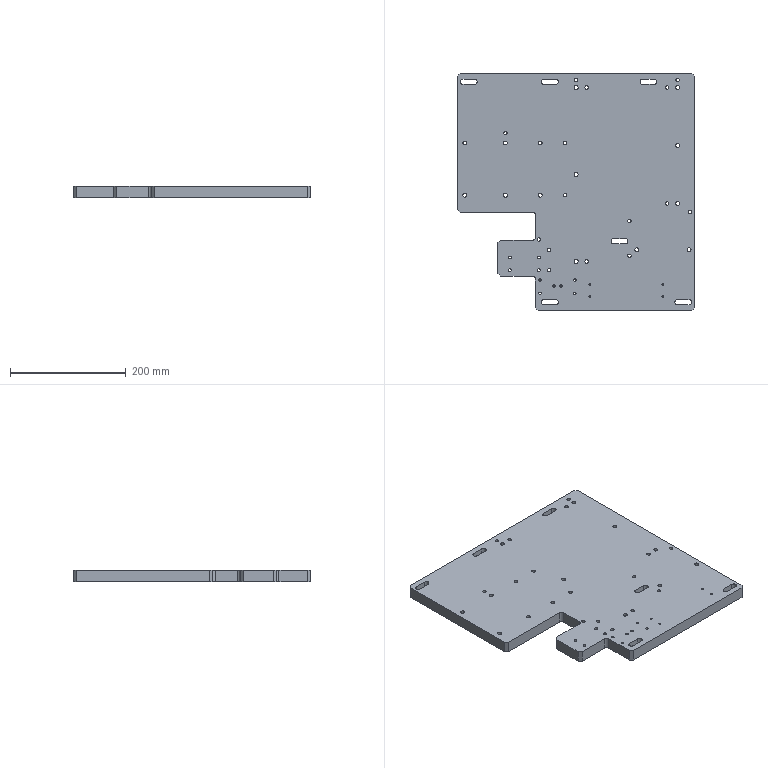Part | 1 solid | 93 faces | box 410 x 410 x 20 mm | volume 2929368 mm3 | cylinder 60 | plane 31 | cone 2 | commonest cylinder face diameters 6 x15 6.8 x14 9 x12 4.2 x6 5 x6 3.3 x4